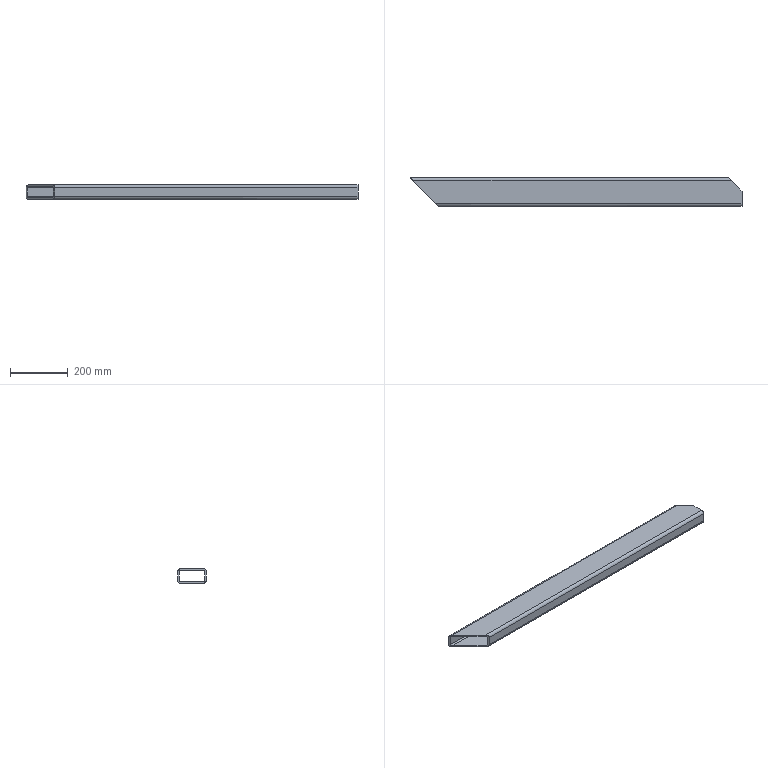Part | SolidWorks | features 3DProfileFeature 1, ICE 1, WeldMemberFeat 1, WeldmentFeature 1 | 1 solid | 19 faces | box 1150 x 100 x 50 mm | volume 1450774 mm3 | plane 11 | cylinder 8 | commonest cylinder face diameters 10 x4 20 x4
STEP:
#1=CARTESIAN_POINT('',(1103.087,50.,-15.));
#2=VERTEX_POINT('',#1);
#3=CARTESIAN_POINT('',(0.,50.,-15.));
#4=VERTEX_POINT('',#3);
#5=CARTESIAN_POINT('',(1150.,50.,-15.));
#6=DIRECTION('',(-1.,0.,0.));
#7=VECTOR('',#6,1000.);
#8=LINE('',#5,#7);
#9=EDGE_CURVE('',#2,#4,#8,.T.);
#10=ORIENTED_EDGE('',*,*,#9,.F.);
#11=CARTESIAN_POINT('',(1113.087,40.,-25.));
#12=VERTEX_POINT('',#11);
#13=CARTESIAN_POINT('',(1103.087,50.,-15.));
#14=CARTESIAN_POINT('',(1103.087,50.,-20.858));
#15=CARTESIAN_POINT('',(1107.229,45.858,-25.));
#16=CARTESIAN_POINT('',(1113.087,40.,-25.));
#17=(BOUNDED_CURVE()B_SPLINE_CURVE(3,(#13,#14,#15,#16),.UNSPECIFIED.,.F.,.F.)B_SPLINE_CURVE_WITH_KNOTS((4,4),(0.,1.571),.UNSPECIFIED.)CURVE()GEOMETRIC_REPRESENTATION_ITEM()RATIONAL_B_SPLINE_CURVE((1.,0.8047,0.8047,1.))REPRESENTATION_ITEM(''));
#18=EDGE_CURVE('',#2,#12,#17,.T.);
#19=ORIENTED_EDGE('',*,*,#18,.T.);
#20=CARTESIAN_POINT('',(10.,40.,-25.));
#21=VERTEX_POINT('',#20);
#22=CARTESIAN_POINT('',(1150.,40.,-25.));
#23=DIRECTION('',(-1.,0.,0.));
#24=VECTOR('',#23,1000.);
#25=LINE('',#22,#24);
#26=EDGE_CURVE('',#12,#21,#25,.T.);
#27=ORIENTED_EDGE('',*,*,#26,.T.);
#28=CARTESIAN_POINT('',(10.,40.,-25.));
#29=CARTESIAN_POINT('',(4.142,45.858,-25.));
#30=CARTESIAN_POINT('',(0.,50.,-20.858));
#31=CARTESIAN_POINT('',(0.,50.,-15.));
#32=(BOUNDED_CURVE()B_SPLINE_CURVE(3,(#28,#29,#30,#31),.UNSPECIFIED.,.F.,.F.)B_SPLINE_CURVE_WITH_KNOTS((4,4),(4.712,6.283),.UNSPECIFIED.)CURVE()GEOMETRIC_REPRESENTATION_ITEM()RATIONAL_B_SPLINE_CURVE((1.,0.8047,0.8047,1.))REPRESENTATION_ITEM(''));
#33=EDGE_CURVE('',#21,#4,#32,.T.);
#34=ORIENTED_EDGE('',*,*,#33,.T.);
#35=EDGE_LOOP('',(#10,#19,#27,#34));
#36=FACE_OUTER_BOUND('',#35,.T.);
#37=CARTESIAN_POINT('',(1150.,40.,-15.));
#38=DIRECTION('',(-1.,0.,0.));
#39=DIRECTION('',(0.,0.,1.));
#40=AXIS2_PLACEMENT_3D('',#37,#38,#39);
#41=CYLINDRICAL_SURFACE('',#40,10.);
#42=ADVANCED_FACE('',(#36),#41,.T.);
#43=CARTESIAN_POINT('',(1103.087,50.,15.));
#44=VERTEX_POINT('',#43);
#45=CARTESIAN_POINT('',(0.,50.,15.));
#46=VERTEX_POINT('',#45);
#47=CARTESIAN_POINT('',(1150.,50.,15.));
#48=DIRECTION('',(-1.,0.,0.));
#49=VECTOR('',#48,1000.);
#50=LINE('',#47,#49);
#51=EDGE_CURVE('',#44,#46,#50,.T.);
#52=ORIENTED_EDGE('',*,*,#51,.F.);
#53=CARTESIAN_POINT('',(1103.087,50.,-166.421));
#54=DIRECTION('',(0.,0.,1.));
#55=VECTOR('',#54,1000.);
#56=LINE('',#53,#55);
#57=EDGE_CURVE('',#2,#44,#56,.T.);
#58=ORIENTED_EDGE('',*,*,#57,.F.);
#59=ORIENTED_EDGE('',*,*,#9,.T.);
#60=CARTESIAN_POINT('',(0.,50.,-15.));
#61=DIRECTION('',(0.,0.,1.));
#62=VECTOR('',#61,1000.);
#63=LINE('',#60,#62);
#64=EDGE_CURVE('',#4,#46,#63,.T.);
#65=ORIENTED_EDGE('',*,*,#64,.T.);
#66=EDGE_LOOP('',(#52,#58,#59,#65));
#67=FACE_OUTER_BOUND('',#66,.T.);
#68=CARTESIAN_POINT('',(1150.,50.,-15.));
#69=DIRECTION('',(0.,-1.,0.));
#70=DIRECTION('',(0.,0.,-1.));
#71=AXIS2_PLACEMENT_3D('',#68,#69,#70);
#72=PLANE('',#71);
#73=ADVANCED_FACE('',(#67),#72,.F.);
#74=CARTESIAN_POINT('',(1113.087,40.,25.));
#75=VERTEX_POINT('',#74);
#76=CARTESIAN_POINT('',(10.,40.,25.));
#77=VERTEX_POINT('',#76);
#78=CARTESIAN_POINT('',(1150.,40.,25.));
#79=DIRECTION('',(-1.,0.,0.));
#80=VECTOR('',#79,1000.);
#81=LINE('',#78,#80);
#82=EDGE_CURVE('',#75,#77,#81,.T.);
#83=ORIENTED_EDGE('',*,*,#82,.F.);
#84=CARTESIAN_POINT('',(1113.087,40.,25.));
#85=CARTESIAN_POINT('',(1107.229,45.858,25.));
#86=CARTESIAN_POINT('',(1103.087,50.,20.858));
#87=CARTESIAN_POINT('',(1103.087,50.,15.));
#88=(BOUNDED_CURVE()B_SPLINE_CURVE(3,(#84,#85,#86,#87),.UNSPECIFIED.,.F.,.T.)B_SPLINE_CURVE_WITH_KNOTS((4,4),(4.712,6.283),.UNSPECIFIED.)CURVE()GEOMETRIC_REPRESENTATION_ITEM()RATIONAL_B_SPLINE_CURVE((1.,0.8047,0.8047,1.))REPRESENTATION_ITEM(''));
#89=EDGE_CURVE('',#75,#44,#88,.T.);
#90=ORIENTED_EDGE('',*,*,#89,.T.);
#91=ORIENTED_EDGE('',*,*,#51,.T.);
#92=CARTESIAN_POINT('',(0.,50.,15.));
#93=CARTESIAN_POINT('',(0.,50.,20.858));
#94=CARTESIAN_POINT('',(4.142,45.858,25.));
#95=CARTESIAN_POINT('',(10.,40.,25.));
#96=(BOUNDED_CURVE()B_SPLINE_CURVE(3,(#92,#93,#94,#95),.UNSPECIFIED.,.F.,.F.)B_SPLINE_CURVE_WITH_KNOTS((4,4),(0.,1.571),.UNSPECIFIED.)CURVE()GEOMETRIC_REPRESENTATION_ITEM()RATIONAL_B_SPLINE_CURVE((1.,0.8047,0.8047,1.))REPRESENTATION_ITEM(''));
#97=EDGE_CURVE('',#46,#77,#96,.T.);
#98=ORIENTED_EDGE('',*,*,#97,.T.);
#99=EDGE_LOOP('',(#83,#90,#91,#98));
#100=FACE_OUTER_BOUND('',#99,.T.);
#101=CARTESIAN_POINT('',(1150.,40.,15.));
#102=DIRECTION('',(-1.,0.,0.));
#103=DIRECTION('',(0.,0.,1.));
#104=AXIS2_PLACEMENT_3D('',#101,#102,#103);
#105=CYLINDRICAL_SURFACE('',#104,10.);
#106=ADVANCED_FACE('',(#100),#105,.T.);
#107=CARTESIAN_POINT('',(1150.,3.087,25.));
#108=VERTEX_POINT('',#107);
#109=CARTESIAN_POINT('',(1150.,-40.,25.));
#110=VERTEX_POINT('',#109);
#111=CARTESIAN_POINT('',(1150.,-40.,25.));
#112=DIRECTION('',(0.,-1.,0.));
#113=VECTOR('',#112,1000.);
#114=LINE('',#111,#113);
#115=EDGE_CURVE('',#108,#110,#114,.T.);
#116=ORIENTED_EDGE('',*,*,#115,.F.);
#117=CARTESIAN_POINT('',(1150.,3.087,25.));
#118=DIRECTION('',(0.7071,-0.7071,0.));
#119=VECTOR('',#118,1000.);
#120=LINE('',#117,#119);
#121=EDGE_CURVE('',#75,#108,#120,.T.);
#122=ORIENTED_EDGE('',*,*,#121,.F.);
#123=ORIENTED_EDGE('',*,*,#82,.T.);
#124=CARTESIAN_POINT('',(90.,-40.,25.));
#125=VERTEX_POINT('',#124);
#126=CARTESIAN_POINT('',(0.,50.,25.));
#127=DIRECTION('',(-0.7071,0.7071,0.));
#128=VECTOR('',#127,1000.);
#129=LINE('',#126,#128);
#130=EDGE_CURVE('',#125,#77,#129,.T.);
#131=ORIENTED_EDGE('',*,*,#130,.F.);
#132=CARTESIAN_POINT('',(1150.,-40.,25.));
#133=DIRECTION('',(-1.,0.,0.));
#134=VECTOR('',#133,1000.);
#135=LINE('',#132,#134);
#136=EDGE_CURVE('',#110,#125,#135,.T.);
#137=ORIENTED_EDGE('',*,*,#136,.F.);
#138=EDGE_LOOP('',(#116,#122,#123,#131,#137));
#139=FACE_OUTER_BOUND('',#138,.T.);
#140=CARTESIAN_POINT('',(1150.,-40.,25.));
#141=DIRECTION('',(0.,0.,-1.));
#142=DIRECTION('',(-1.,0.,0.));
#143=AXIS2_PLACEMENT_3D('',#140,#141,#142);
#144=PLANE('',#143);
#145=ADVANCED_FACE('',(#139),#144,.F.);
#146=ORIENTED_EDGE('',*,*,#136,.T.);
#147=CARTESIAN_POINT('',(100.,-50.,15.));
#148=VERTEX_POINT('',#147);
#149=CARTESIAN_POINT('',(90.,-40.,25.));
#150=CARTESIAN_POINT('',(95.858,-45.858,25.));
#151=CARTESIAN_POINT('',(100.,-50.,20.858));
#152=CARTESIAN_POINT('',(100.,-50.,15.));
#153=(BOUNDED_CURVE()B_SPLINE_CURVE(3,(#149,#150,#151,#152),.UNSPECIFIED.,.F.,.F.)B_SPLINE_CURVE_WITH_KNOTS((4,4),(1.571,3.142),.UNSPECIFIED.)CURVE()GEOMETRIC_REPRESENTATION_ITEM()RATIONAL_B_SPLINE_CURVE((1.,0.8047,0.8047,1.))REPRESENTATION_ITEM(''));
#154=EDGE_CURVE('',#125,#148,#153,.T.);
#155=ORIENTED_EDGE('',*,*,#154,.T.);
#156=CARTESIAN_POINT('',(1150.,-50.,15.));
#157=VERTEX_POINT('',#156);
#158=CARTESIAN_POINT('',(1150.,-50.,15.));
#159=DIRECTION('',(-1.,0.,0.));
#160=VECTOR('',#159,1000.);
#161=LINE('',#158,#160);
#162=EDGE_CURVE('',#157,#148,#161,.T.);
#163=ORIENTED_EDGE('',*,*,#162,.F.);
#164=CARTESIAN_POINT('',(1150.,-40.,15.));
#165=DIRECTION('',(1.,0.,0.));
#166=DIRECTION('',(0.,0.,-1.));
#167=AXIS2_PLACEMENT_3D('',#164,#165,#166);
#168=CIRCLE('',#167,10.);
#169=EDGE_CURVE('',#110,#157,#168,.T.);
#170=ORIENTED_EDGE('',*,*,#169,.F.);
#171=EDGE_LOOP('',(#146,#155,#163,#170));
#172=FACE_OUTER_BOUND('',#171,.T.);
#173=CARTESIAN_POINT('',(1150.,-40.,15.));
#174=DIRECTION('',(-1.,0.,0.));
#175=DIRECTION('',(0.,0.,1.));
#176=AXIS2_PLACEMENT_3D('',#173,#174,#175);
#177=CYLINDRICAL_SURFACE('',#176,10.);
#178=ADVANCED_FACE('',(#172),#177,.T.);
#179=ORIENTED_EDGE('',*,*,#162,.T.);
#180=CARTESIAN_POINT('',(100.,-50.,-15.));
#181=VERTEX_POINT('',#180);
#182=CARTESIAN_POINT('',(100.,-50.,-166.421));
#183=DIRECTION('',(0.,0.,1.));
#184=VECTOR('',#183,1000.);
#185=LINE('',#182,#184);
#186=EDGE_CURVE('',#181,#148,#185,.T.);
#187=ORIENTED_EDGE('',*,*,#186,.F.);
#188=CARTESIAN_POINT('',(1150.,-50.,-15.));
#189=VERTEX_POINT('',#188);
#190=CARTESIAN_POINT('',(1150.,-50.,-15.));
#191=DIRECTION('',(-1.,0.,0.));
#192=VECTOR('',#191,1000.);
#193=LINE('',#190,#192);
#194=EDGE_CURVE('',#189,#181,#193,.T.);
#195=ORIENTED_EDGE('',*,*,#194,.F.);
#196=CARTESIAN_POINT('',(1150.,-50.,15.));
#197=DIRECTION('',(0.,0.,-1.));
#198=VECTOR('',#197,1000.);
#199=LINE('',#196,#198);
#200=EDGE_CURVE('',#157,#189,#199,.T.);
#201=ORIENTED_EDGE('',*,*,#200,.F.);
#202=EDGE_LOOP('',(#179,#187,#195,#201));
#203=FACE_OUTER_BOUND('',#202,.T.);
#204=CARTESIAN_POINT('',(1150.,-50.,15.));
#205=DIRECTION('',(0.,1.,0.));
#206=DIRECTION('',(0.,0.,1.));
#207=AXIS2_PLACEMENT_3D('',#204,#205,#206);
#208=PLANE('',#207);
#209=ADVANCED_FACE('',(#203),#208,.F.);
#210=ORIENTED_EDGE('',*,*,#194,.T.);
#211=CARTESIAN_POINT('',(90.,-40.,-25.));
#212=VERTEX_POINT('',#211);
#213=CARTESIAN_POINT('',(100.,-50.,-15.));
#214=CARTESIAN_POINT('',(100.,-50.,-20.858));
#215=CARTESIAN_POINT('',(95.858,-45.858,-25.));
#216=CARTESIAN_POINT('',(90.,-40.,-25.));
#217=(BOUNDED_CURVE()B_SPLINE_CURVE(3,(#213,#214,#215,#216),.UNSPECIFIED.,.F.,.F.)B_SPLINE_CURVE_WITH_KNOTS((4,4),(3.142,4.712),.UNSPECIFIED.)CURVE()GEOMETRIC_REPRESENTATION_ITEM()RATIONAL_B_SPLINE_CURVE((1.,0.8047,0.8047,1.))REPRESENTATION_ITEM(''));
#218=EDGE_CURVE('',#181,#212,#217,.T.);
#219=ORIENTED_EDGE('',*,*,#218,.T.);
#220=CARTESIAN_POINT('',(1150.,-40.,-25.));
#221=VERTEX_POINT('',#220);
#222=CARTESIAN_POINT('',(1150.,-40.,-25.));
#223=DIRECTION('',(-1.,0.,0.));
#224=VECTOR('',#223,1000.);
#225=LINE('',#222,#224);
#226=EDGE_CURVE('',#221,#212,#225,.T.);
#227=ORIENTED_EDGE('',*,*,#226,.F.);
#228=CARTESIAN_POINT('',(1150.,-40.,-15.));
#229=DIRECTION('',(1.,0.,0.));
#230=DIRECTION('',(0.,0.,-1.));
#231=AXIS2_PLACEMENT_3D('',#228,#229,#230);
#232=CIRCLE('',#231,10.);
#233=EDGE_CURVE('',#189,#221,#232,.T.);
#234=ORIENTED_EDGE('',*,*,#233,.F.);
#235=EDGE_LOOP('',(#210,#219,#227,#234));
#236=FACE_OUTER_BOUND('',#235,.T.);
#237=CARTESIAN_POINT('',(1150.,-40.,-15.));
#238=DIRECTION('',(-1.,0.,0.));
#239=DIRECTION('',(0.,0.,1.));
#240=AXIS2_PLACEMENT_3D('',#237,#238,#239);
#241=CYLINDRICAL_SURFACE('',#240,10.);
#242=ADVANCED_FACE('',(#236),#241,.T.);
#243=CARTESIAN_POINT('',(1113.087,40.,20.));
#244=VERTEX_POINT('',#243);
#245=CARTESIAN_POINT('',(1108.087,45.,15.));
#246=VERTEX_POINT('',#245);
#247=CARTESIAN_POINT('',(1113.087,40.,20.));
#248=CARTESIAN_POINT('',(1110.158,42.929,20.));
#249=CARTESIAN_POINT('',(1108.087,45.,17.929));
#250=CARTESIAN_POINT('',(1108.087,45.,15.));
#251=(BOUNDED_CURVE()B_SPLINE_CURVE(3,(#247,#248,#249,#250),.UNSPECIFIED.,.F.,.F.)B_SPLINE_CURVE_WITH_KNOTS((4,4),(4.712,6.283),.UNSPECIFIED.)CURVE()GEOMETRIC_REPRESENTATION_ITEM()RATIONAL_B_SPLINE_CURVE((1.,0.8047,0.8047,1.))REPRESENTATION_ITEM(''));
#252=EDGE_CURVE('',#244,#246,#251,.T.);
#253=ORIENTED_EDGE('',*,*,#252,.F.);
#254=CARTESIAN_POINT('',(10.,40.,20.));
#255=VERTEX_POINT('',#254);
#256=CARTESIAN_POINT('',(1150.,40.,20.));
#257=DIRECTION('',(-1.,0.,0.));
#258=VECTOR('',#257,1000.);
#259=LINE('',#256,#258);
#260=EDGE_CURVE('',#244,#255,#259,.T.);
#261=ORIENTED_EDGE('',*,*,#260,.T.);
#262=CARTESIAN_POINT('',(5.,45.,15.));
#263=VERTEX_POINT('',#262);
#264=CARTESIAN_POINT('',(5.,45.,15.));
#265=CARTESIAN_POINT('',(5.,45.,17.929));
#266=CARTESIAN_POINT('',(7.071,42.929,20.));
#267=CARTESIAN_POINT('',(10.,40.,20.));
#268=(BOUNDED_CURVE()B_SPLINE_CURVE(3,(#264,#265,#266,#267),.UNSPECIFIED.,.F.,.F.)B_SPLINE_CURVE_WITH_KNOTS((4,4),(0.,1.571),.UNSPECIFIED.)CURVE()GEOMETRIC_REPRESENTATION_ITEM()RATIONAL_B_SPLINE_CURVE((1.,0.8047,0.8047,1.))REPRESENTATION_ITEM(''));
#269=EDGE_CURVE('',#263,#255,#268,.T.);
#270=ORIENTED_EDGE('',*,*,#269,.F.);
#271=CARTESIAN_POINT('',(1150.,45.,15.));
#272=DIRECTION('',(-1.,0.,0.));
#273=VECTOR('',#272,1000.);
#274=LINE('',#271,#273);
#275=EDGE_CURVE('',#246,#263,#274,.T.);
#276=ORIENTED_EDGE('',*,*,#275,.F.);
#277=EDGE_LOOP('',(#253,#261,#270,#276));
#278=FACE_OUTER_BOUND('',#277,.T.);
#279=CARTESIAN_POINT('',(1150.,40.,15.));
#280=DIRECTION('',(-1.,0.,0.));
#281=DIRECTION('',(0.,0.,1.));
#282=AXIS2_PLACEMENT_3D('',#279,#280,#281);
#283=CYLINDRICAL_SURFACE('',#282,5.);
#284=ADVANCED_FACE('',(#278),#283,.F.);
#285=CARTESIAN_POINT('',(1108.087,45.,-15.));
#286=VERTEX_POINT('',#285);
#287=CARTESIAN_POINT('',(1108.087,45.,-15.));
#288=DIRECTION('',(0.,0.,-1.));
#289=VECTOR('',#288,1000.);
#290=LINE('',#287,#289);
#291=EDGE_CURVE('',#246,#286,#290,.T.);
#292=ORIENTED_EDGE('',*,*,#291,.F.);
#293=ORIENTED_EDGE('',*,*,#275,.T.);
#294=CARTESIAN_POINT('',(5.,45.,-15.));
#295=VERTEX_POINT('',#294);
#296=CARTESIAN_POINT('',(5.,45.,-15.));
#297=DIRECTION('',(0.,0.,1.));
#298=VECTOR('',#297,1000.);
#299=LINE('',#296,#298);
#300=EDGE_CURVE('',#295,#263,#299,.T.);
#301=ORIENTED_EDGE('',*,*,#300,.F.);
#302=CARTESIAN_POINT('',(1150.,45.,-15.));
#303=DIRECTION('',(-1.,0.,0.));
#304=VECTOR('',#303,1000.);
#305=LINE('',#302,#304);
#306=EDGE_CURVE('',#286,#295,#305,.T.);
#307=ORIENTED_EDGE('',*,*,#306,.F.);
#308=EDGE_LOOP('',(#292,#293,#301,#307));
#309=FACE_OUTER_BOUND('',#308,.T.);
#310=CARTESIAN_POINT('',(1150.,45.,-15.));
#311=DIRECTION('',(0.,-1.,0.));
#312=DIRECTION('',(0.,0.,-1.));
#313=AXIS2_PLACEMENT_3D('',#310,#311,#312);
#314=PLANE('',#313);
#315=ADVANCED_FACE('',(#309),#314,.T.);
#316=CARTESIAN_POINT('',(1113.087,40.,-20.));
#317=VERTEX_POINT('',#316);
#318=CARTESIAN_POINT('',(1108.087,45.,-15.));
#319=CARTESIAN_POINT('',(1108.087,45.,-17.929));
#320=CARTESIAN_POINT('',(1110.158,42.929,-20.));
#321=CARTESIAN_POINT('',(1113.087,40.,-20.));
#322=(BOUNDED_CURVE()B_SPLINE_CURVE(3,(#318,#319,#320,#321),.UNSPECIFIED.,.F.,.T.)B_SPLINE_CURVE_WITH_KNOTS((4,4),(0.,1.571),.UNSPECIFIED.)CURVE()GEOMETRIC_REPRESENTATION_ITEM()RATIONAL_B_SPLINE_CURVE((1.,0.8047,0.8047,1.))REPRESENTATION_ITEM(''));
#323=EDGE_CURVE('',#286,#317,#322,.T.);
#324=ORIENTED_EDGE('',*,*,#323,.F.);
#325=ORIENTED_EDGE('',*,*,#306,.T.);
#326=CARTESIAN_POINT('',(10.,40.,-20.));
#327=VERTEX_POINT('',#326);
#328=CARTESIAN_POINT('',(10.,40.,-20.));
#329=CARTESIAN_POINT('',(7.071,42.929,-20.));
#330=CARTESIAN_POINT('',(5.,45.,-17.929));
#331=CARTESIAN_POINT('',(5.,45.,-15.));
#332=(BOUNDED_CURVE()B_SPLINE_CURVE(3,(#328,#329,#330,#331),.UNSPECIFIED.,.F.,.F.)B_SPLINE_CURVE_WITH_KNOTS((4,4),(4.712,6.283),.UNSPECIFIED.)CURVE()GEOMETRIC_REPRESENTATION_ITEM()RATIONAL_B_SPLINE_CURVE((1.,0.8047,0.8047,1.))REPRESENTATION_ITEM(''));
#333=EDGE_CURVE('',#327,#295,#332,.T.);
#334=ORIENTED_EDGE('',*,*,#333,.F.);
#335=CARTESIAN_POINT('',(1150.,40.,-20.));
#336=DIRECTION('',(-1.,0.,0.));
#337=VECTOR('',#336,1000.);
#338=LINE('',#335,#337);
#339=EDGE_CURVE('',#317,#327,#338,.T.);
#340=ORIENTED_EDGE('',*,*,#339,.F.);
#341=EDGE_LOOP('',(#324,#325,#334,#340));
#342=FACE_OUTER_BOUND('',#341,.T.);
#343=CARTESIAN_POINT('',(1150.,40.,-15.));
#344=DIRECTION('',(-1.,0.,0.));
#345=DIRECTION('',(0.,0.,1.));
#346=AXIS2_PLACEMENT_3D('',#343,#344,#345);
#347=CYLINDRICAL_SURFACE('',#346,5.);
#348=ADVANCED_FACE('',(#342),#347,.F.);
#349=CARTESIAN_POINT('',(1150.,3.087,-20.));
#350=VERTEX_POINT('',#349);
#351=CARTESIAN_POINT('',(1131.543,21.543,-20.));
#352=DIRECTION('',(0.7071,-0.7071,0.));
#353=VECTOR('',#352,1000.);
#354=LINE('',#351,#353);
#355=EDGE_CURVE('',#317,#350,#354,.T.);
#356=ORIENTED_EDGE('',*,*,#355,.F.);
#357=ORIENTED_EDGE('',*,*,#339,.T.);
#358=CARTESIAN_POINT('',(90.,-40.,-20.));
#359=VERTEX_POINT('',#358);
#360=CARTESIAN_POINT('',(580.,-530.,-20.));
#361=DIRECTION('',(-0.7071,0.7071,0.));
#362=VECTOR('',#361,1000.);
#363=LINE('',#360,#362);
#364=EDGE_CURVE('',#359,#327,#363,.T.);
#365=ORIENTED_EDGE('',*,*,#364,.F.);
#366=CARTESIAN_POINT('',(1150.,-40.,-20.));
#367=VERTEX_POINT('',#366);
#368=CARTESIAN_POINT('',(1150.,-40.,-20.));
#369=DIRECTION('',(-1.,0.,0.));
#370=VECTOR('',#369,1000.);
#371=LINE('',#368,#370);
#372=EDGE_CURVE('',#367,#359,#371,.T.);
#373=ORIENTED_EDGE('',*,*,#372,.F.);
#374=CARTESIAN_POINT('',(1150.,40.,-20.));
#375=DIRECTION('',(0.,1.,0.));
#376=VECTOR('',#375,1000.);
#377=LINE('',#374,#376);
#378=EDGE_CURVE('',#367,#350,#377,.T.);
#379=ORIENTED_EDGE('',*,*,#378,.T.);
#380=EDGE_LOOP('',(#356,#357,#365,#373,#379));
#381=FACE_OUTER_BOUND('',#380,.T.);
#382=CARTESIAN_POINT('',(1150.,40.,-20.));
#383=DIRECTION('',(0.,0.,1.));
#384=DIRECTION('',(1.,0.,0.));
#385=AXIS2_PLACEMENT_3D('',#382,#383,#384);
#386=PLANE('',#385);
#387=ADVANCED_FACE('',(#381),#386,.T.);
#388=CARTESIAN_POINT('',(95.,-45.,-15.));
#389=VERTEX_POINT('',#388);
#390=CARTESIAN_POINT('',(95.,-45.,-15.));
#391=CARTESIAN_POINT('',(95.,-45.,-17.929));
#392=CARTESIAN_POINT('',(92.929,-42.929,-20.));
#393=CARTESIAN_POINT('',(90.,-40.,-20.));
#394=(BOUNDED_CURVE()B_SPLINE_CURVE(3,(#390,#391,#392,#393),.UNSPECIFIED.,.F.,.F.)B_SPLINE_CURVE_WITH_KNOTS((4,4),(3.142,4.712),.UNSPECIFIED.)CURVE()GEOMETRIC_REPRESENTATION_ITEM()RATIONAL_B_SPLINE_CURVE((1.,0.8047,0.8047,1.))REPRESENTATION_ITEM(''));
#395=EDGE_CURVE('',#389,#359,#394,.T.);
#396=ORIENTED_EDGE('',*,*,#395,.F.);
#397=CARTESIAN_POINT('',(1150.,-45.,-15.));
#398=VERTEX_POINT('',#397);
#399=CARTESIAN_POINT('',(1150.,-45.,-15.));
#400=DIRECTION('',(-1.,0.,0.));
#401=VECTOR('',#400,1000.);
#402=LINE('',#399,#401);
#403=EDGE_CURVE('',#398,#389,#402,.T.);
#404=ORIENTED_EDGE('',*,*,#403,.F.);
#405=CARTESIAN_POINT('',(1150.,-40.,-15.));
#406=DIRECTION('',(1.,0.,0.));
#407=DIRECTION('',(0.,0.,-1.));
#408=AXIS2_PLACEMENT_3D('',#405,#406,#407);
#409=CIRCLE('',#408,5.);
#410=EDGE_CURVE('',#398,#367,#409,.T.);
#411=ORIENTED_EDGE('',*,*,#410,.T.);
#412=ORIENTED_EDGE('',*,*,#372,.T.);
#413=EDGE_LOOP('',(#396,#404,#411,#412));
#414=FACE_OUTER_BOUND('',#413,.T.);
#415=CARTESIAN_POINT('',(1150.,-40.,-15.));
#416=DIRECTION('',(-1.,0.,0.));
#417=DIRECTION('',(0.,0.,1.));
#418=AXIS2_PLACEMENT_3D('',#415,#416,#417);
#419=CYLINDRICAL_SURFACE('',#418,5.);
#420=ADVANCED_FACE('',(#414),#419,.F.);
#421=CARTESIAN_POINT('',(95.,-45.,15.));
#422=VERTEX_POINT('',#421);
#423=CARTESIAN_POINT('',(95.,-45.,15.));
#424=DIRECTION('',(0.,0.,-1.));
#425=VECTOR('',#424,1000.);
#426=LINE('',#423,#425);
#427=EDGE_CURVE('',#422,#389,#426,.T.);
#428=ORIENTED_EDGE('',*,*,#427,.F.);
#429=CARTESIAN_POINT('',(1150.,-45.,15.));
#430=VERTEX_POINT('',#429);
#431=CARTESIAN_POINT('',(1150.,-45.,15.));
#432=DIRECTION('',(-1.,0.,0.));
#433=VECTOR('',#432,1000.);
#434=LINE('',#431,#433);
#435=EDGE_CURVE('',#430,#422,#434,.T.);
#436=ORIENTED_EDGE('',*,*,#435,.F.);
#437=CARTESIAN_POINT('',(1150.,-45.,15.));
#438=DIRECTION('',(0.,0.,-1.));
#439=VECTOR('',#438,1000.);
#440=LINE('',#437,#439);
#441=EDGE_CURVE('',#430,#398,#440,.T.);
#442=ORIENTED_EDGE('',*,*,#441,.T.);
#443=ORIENTED_EDGE('',*,*,#403,.T.);
#444=EDGE_LOOP('',(#428,#436,#442,#443));
#445=FACE_OUTER_BOUND('',#444,.T.);
#446=CARTESIAN_POINT('',(1150.,-45.,15.));
#447=DIRECTION('',(0.,1.,0.));
#448=DIRECTION('',(0.,0.,1.));
#449=AXIS2_PLACEMENT_3D('',#446,#447,#448);
#450=PLANE('',#449);
#451=ADVANCED_FACE('',(#445),#450,.T.);
#452=CARTESIAN_POINT('',(90.,-40.,20.));
#453=VERTEX_POINT('',#452);
#454=CARTESIAN_POINT('',(90.,-40.,20.));
#455=CARTESIAN_POINT('',(92.929,-42.929,20.));
#456=CARTESIAN_POINT('',(95.,-45.,17.929));
#457=CARTESIAN_POINT('',(95.,-45.,15.));
#458=(BOUNDED_CURVE()B_SPLINE_CURVE(3,(#454,#455,#456,#457),.UNSPECIFIED.,.F.,.F.)B_SPLINE_CURVE_WITH_KNOTS((4,4),(1.571,3.142),.UNSPECIFIED.)CURVE()GEOMETRIC_REPRESENTATION_ITEM()RATIONAL_B_SPLINE_CURVE((1.,0.8047,0.8047,1.))REPRESENTATION_ITEM(''));
#459=EDGE_CURVE('',#453,#422,#458,.T.);
#460=ORIENTED_EDGE('',*,*,#459,.F.);
#461=CARTESIAN_POINT('',(1150.,-40.,20.));
#462=VERTEX_POINT('',#461);
#463=CARTESIAN_POINT('',(1150.,-40.,20.));
#464=DIRECTION('',(-1.,0.,0.));
#465=VECTOR('',#464,1000.);
#466=LINE('',#463,#465);
#467=EDGE_CURVE('',#462,#453,#466,.T.);
#468=ORIENTED_EDGE('',*,*,#467,.F.);
#469=CARTESIAN_POINT('',(1150.,-40.,15.));
#470=DIRECTION('',(1.,0.,0.));
#471=DIRECTION('',(0.,0.,-1.));
#472=AXIS2_PLACEMENT_3D('',#469,#470,#471);
#473=CIRCLE('',#472,5.);
#474=EDGE_CURVE('',#462,#430,#473,.T.);
#475=ORIENTED_EDGE('',*,*,#474,.T.);
#476=ORIENTED_EDGE('',*,*,#435,.T.);
#477=EDGE_LOOP('',(#460,#468,#475,#476));
#478=FACE_OUTER_BOUND('',#477,.T.);
#479=CARTESIAN_POINT('',(1150.,-40.,15.));
#480=DIRECTION('',(-1.,0.,0.));
#481=DIRECTION('',(0.,0.,1.));
#482=AXIS2_PLACEMENT_3D('',#479,#480,#481);
#483=CYLINDRICAL_SURFACE('',#482,5.);
#484=ADVANCED_FACE('',(#478),#483,.F.);
#485=CARTESIAN_POINT('',(1150.,3.087,20.));
#486=VERTEX_POINT('',#485);
#487=CARTESIAN_POINT('',(1171.543,-18.457,20.));
#488=DIRECTION('',(-0.7071,0.7071,0.));
#489=VECTOR('',#488,1000.);
#490=LINE('',#487,#489);
#491=EDGE_CURVE('',#486,#244,#490,.T.);
#492=ORIENTED_EDGE('',*,*,#491,.F.);
#493=CARTESIAN_POINT('',(1150.,-40.,20.));
#494=DIRECTION('',(0.,-1.,0.));
#495=VECTOR('',#494,1000.);
#496=LINE('',#493,#495);
#497=EDGE_CURVE('',#486,#462,#496,.T.);
#498=ORIENTED_EDGE('',*,*,#497,.T.);
#499=ORIENTED_EDGE('',*,*,#467,.T.);
#500=CARTESIAN_POINT('',(620.,-570.,20.));
#501=DIRECTION('',(0.7071,-0.7071,0.));
#502=VECTOR('',#501,1000.);
#503=LINE('',#500,#502);
#504=EDGE_CURVE('',#255,#453,#503,.T.);
#505=ORIENTED_EDGE('',*,*,#504,.F.);
#506=ORIENTED_EDGE('',*,*,#260,.F.);
#507=EDGE_LOOP('',(#492,#498,#499,#505,#506));
#508=FACE_OUTER_BOUND('',#507,.T.);
#509=CARTESIAN_POINT('',(1150.,-40.,20.));
#510=DIRECTION('',(0.,0.,-1.));
#511=DIRECTION('',(-1.,0.,0.));
#512=AXIS2_PLACEMENT_3D('',#509,#510,#511);
#513=PLANE('',#512);
#514=ADVANCED_FACE('',(#508),#513,.T.);
#515=ORIENTED_EDGE('',*,*,#26,.F.);
#516=CARTESIAN_POINT('',(1150.,3.087,-25.));
#517=VERTEX_POINT('',#516);
#518=CARTESIAN_POINT('',(1150.,3.087,-25.));
#519=DIRECTION('',(-0.7071,0.7071,0.));
#520=VECTOR('',#519,1000.);
#521=LINE('',#518,#520);
#522=EDGE_CURVE('',#517,#12,#521,.T.);
#523=ORIENTED_EDGE('',*,*,#522,.F.);
#524=CARTESIAN_POINT('',(1150.,40.,-25.));
#525=DIRECTION('',(0.,1.,0.));
#526=VECTOR('',#525,1000.);
#527=LINE('',#524,#526);
#528=EDGE_CURVE('',#221,#517,#527,.T.);
#529=ORIENTED_EDGE('',*,*,#528,.F.);
#530=ORIENTED_EDGE('',*,*,#226,.T.);
#531=CARTESIAN_POINT('',(0.,50.,-25.));
#532=DIRECTION('',(0.7071,-0.7071,0.));
#533=VECTOR('',#532,1000.);
#534=LINE('',#531,#533);
#535=EDGE_CURVE('',#21,#212,#534,.T.);
#536=ORIENTED_EDGE('',*,*,#535,.F.);
#537=EDGE_LOOP('',(#515,#523,#529,#530,#536));
#538=FACE_OUTER_BOUND('',#537,.T.);
#539=CARTESIAN_POINT('',(1150.,40.,-25.));
#540=DIRECTION('',(0.,0.,1.));
#541=DIRECTION('',(1.,0.,0.));
#542=AXIS2_PLACEMENT_3D('',#539,#540,#541);
#543=PLANE('',#542);
#544=ADVANCED_FACE('',(#538),#543,.F.);
#545=CARTESIAN_POINT('',(1150.,3.087,-15.));
#546=DIRECTION('',(0.,0.,-1.));
#547=VECTOR('',#546,1000.);
#548=LINE('',#545,#547);
#549=EDGE_CURVE('',#108,#486,#548,.T.);
#550=ORIENTED_EDGE('',*,*,#549,.F.);
#551=ORIENTED_EDGE('',*,*,#115,.T.);
#552=ORIENTED_EDGE('',*,*,#169,.T.);
#553=ORIENTED_EDGE('',*,*,#200,.T.);
#554=ORIENTED_EDGE('',*,*,#233,.T.);
#555=ORIENTED_EDGE('',*,*,#528,.T.);
#556=CARTESIAN_POINT('',(1150.,3.087,-166.421));
#557=DIRECTION('',(0.,0.,1.));
#558=VECTOR('',#557,1000.);
#559=LINE('',#556,#558);
#560=EDGE_CURVE('',#517,#350,#559,.T.);
#561=ORIENTED_EDGE('',*,*,#560,.T.);
#562=ORIENTED_EDGE('',*,*,#378,.F.);
#563=ORIENTED_EDGE('',*,*,#410,.F.);
#564=ORIENTED_EDGE('',*,*,#441,.F.);
#565=ORIENTED_EDGE('',*,*,#474,.F.);
#566=ORIENTED_EDGE('',*,*,#497,.F.);
#567=EDGE_LOOP('',(#550,#551,#552,#553,#554,#555,#561,#562,#563,#564,#565,#566));
#568=FACE_OUTER_BOUND('',#567,.T.);
#569=CARTESIAN_POINT('',(1150.,40.,-15.));
#570=DIRECTION('',(1.,0.,0.));
#571=DIRECTION('',(0.,0.,-1.));
#572=AXIS2_PLACEMENT_3D('',#569,#570,#571);
#573=PLANE('',#572);
#574=ADVANCED_FACE('',(#568),#573,.T.);
#575=ORIENTED_EDGE('',*,*,#269,.T.);
#576=ORIENTED_EDGE('',*,*,#504,.T.);
#577=ORIENTED_EDGE('',*,*,#459,.T.);
#578=ORIENTED_EDGE('',*,*,#427,.T.);
#579=ORIENTED_EDGE('',*,*,#395,.T.);
#580=ORIENTED_EDGE('',*,*,#364,.T.);
#581=ORIENTED_EDGE('',*,*,#333,.T.);
#582=ORIENTED_EDGE('',*,*,#300,.T.);
#583=EDGE_LOOP('',(#575,#576,#577,#578,#579,#580,#581,#582));
#584=FACE_BOUND('',#583,.T.);
#585=ORIENTED_EDGE('',*,*,#535,.T.);
#586=ORIENTED_EDGE('',*,*,#218,.F.);
#587=ORIENTED_EDGE('',*,*,#186,.T.);
#588=ORIENTED_EDGE('',*,*,#154,.F.);
#589=ORIENTED_EDGE('',*,*,#130,.T.);
#590=ORIENTED_EDGE('',*,*,#97,.F.);
#591=ORIENTED_EDGE('',*,*,#64,.F.);
#592=ORIENTED_EDGE('',*,*,#33,.F.);
#593=EDGE_LOOP('',(#585,#586,#587,#588,#589,#590,#591,#592));
#594=FACE_OUTER_BOUND('',#593,.T.);
#595=CARTESIAN_POINT('',(0.,50.,-166.421));
#596=DIRECTION('',(0.7071,0.7071,0.));
#597=DIRECTION('',(-0.7071,0.7071,0.));
#598=AXIS2_PLACEMENT_3D('',#595,#596,#597);
#599=PLANE('',#598);
#600=ADVANCED_FACE('',(#584,#594),#599,.F.);
#601=ORIENTED_EDGE('',*,*,#57,.T.);
#602=ORIENTED_EDGE('',*,*,#89,.F.);
#603=ORIENTED_EDGE('',*,*,#121,.T.);
#604=ORIENTED_EDGE('',*,*,#549,.T.);
#605=ORIENTED_EDGE('',*,*,#491,.T.);
#606=ORIENTED_EDGE('',*,*,#252,.T.);
#607=ORIENTED_EDGE('',*,*,#291,.T.);
#608=ORIENTED_EDGE('',*,*,#323,.T.);
#609=ORIENTED_EDGE('',*,*,#355,.T.);
#610=ORIENTED_EDGE('',*,*,#560,.F.);
#611=ORIENTED_EDGE('',*,*,#522,.T.);
#612=ORIENTED_EDGE('',*,*,#18,.F.);
#613=EDGE_LOOP('',(#601,#602,#603,#604,#605,#606,#607,#608,#609,#610,#611,#612));
#614=FACE_OUTER_BOUND('',#613,.T.);
#615=CARTESIAN_POINT('',(1150.,3.087,-166.421));
#616=DIRECTION('',(-0.7071,-0.7071,0.));
#617=DIRECTION('',(0.7071,-0.7071,0.));
#618=AXIS2_PLACEMENT_3D('',#615,#616,#617);
#619=PLANE('',#618);
#620=ADVANCED_FACE('',(#614),#619,.F.);
#621=CLOSED_SHELL('',(#42,#73,#106,#145,#178,#209,#242,#284,#315,#348,#387,#420,#451,#484,#514,#544,#574,#600,#620));
#622=MANIFOLD_SOLID_BREP('',#621);
#623=CARTESIAN_POINT('',(0.,0.,0.));
#624=DIRECTION('',(0.,0.,1.));
#625=DIRECTION('',(1.,0.,0.));
#626=AXIS2_PLACEMENT_3D('',#623,#624,#625);
#627=(LENGTH_UNIT()NAMED_UNIT(*)SI_UNIT(.MILLI.,.METRE.));
#628=UNCERTAINTY_MEASURE_WITH_UNIT(LENGTH_MEASURE(0.00001),#627,'','');
#629=(NAMED_UNIT(*)PLANE_ANGLE_UNIT()SI_UNIT($,.RADIAN.));
#630=(NAMED_UNIT(*)SI_UNIT($,.STERADIAN.)SOLID_ANGLE_UNIT());
#631=(GEOMETRIC_REPRESENTATION_CONTEXT(3)GLOBAL_UNCERTAINTY_ASSIGNED_CONTEXT((#628))GLOBAL_UNIT_ASSIGNED_CONTEXT((#627,#629,#630))REPRESENTATION_CONTEXT('',''));
#632=ADVANCED_BREP_SHAPE_REPRESENTATION('',(#622,#626),#631);